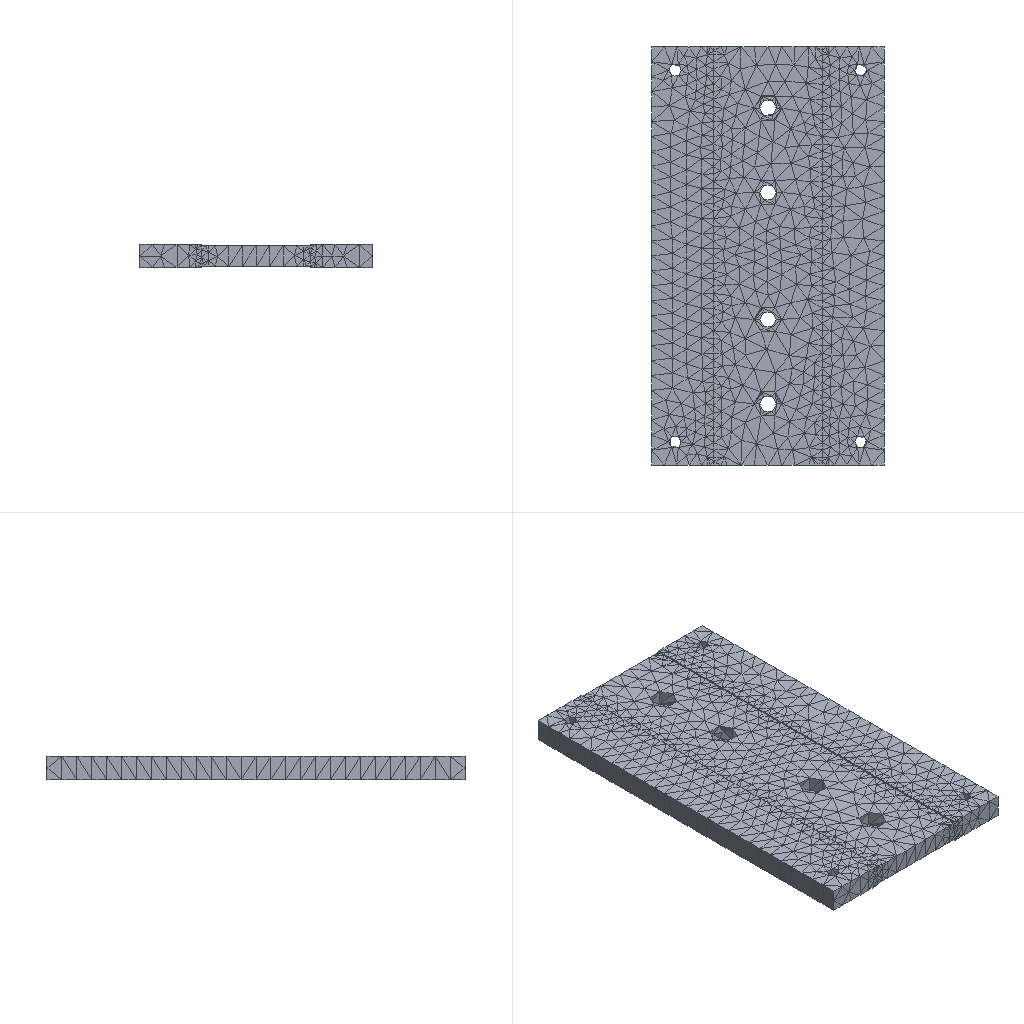Simulation study | ansys workbench
Set-up summary:
category,name,step,type,value,unit,region
solver,ansys_workbench
units,SI m-kg-s (Pa),,stated,"/units,MKS"
analysis,LS1,,static
load_step,LS1,LS1,static,nsubst=1; time=1
mesh,nodes,,,15924
mesh,elements,,,9787
element_type,SOLID187,,,9141
element_type,CONTA174,,,646
material,Structural Steel,,E,2e+11,Pa
material,Structural Steel,,nu,0.3
material,Structural Steel,,density,7850,kg m^-3
material,Structural Steel,,conductivity,60.5,W m^-1 C^-1
material,Structural Steel,,specific_heat,434,J kg^-1 C^-1
material,Structural Steel,,cte,1.2e-05,C^-1
material,Structural Steel,,permeability,10000
material,Structural Steel,,resistivity,1.7e-07,kg m^3 A^-2 s^-3
load,,LS1,moment,"1000 [dir=(0, 0, 1) n=3]",,all
bc,Fixed Supports,model,fixed,[dofs=ALL],,_FIXEDSU
contact,contact 1,,bonded (always),element=CONTA174
named_set,_FIXEDSU,,node,1510
Ansys APDL input file, long lists of numbers shortened:
/batch
/config,noeldb,1     ! force off writing results to database
*get,_wallstrt,active,,time,wall
! ANSYS input file written by Workbench version 2024 R1
! File used for geometry attach:
/title,wbnew--____ (A5)
! ****** Begin Custom Load Command Snippet ******
/COM, ACT Extensions:
/COM,     LSDYNA, 2024.1
/COM,/COM,     ANSYSMotion, 2024.1
/COM,
! ****** End   Custom Load Command Snippet ******
*DIM,_wb_ProjectScratch_dir,string,248
_wb_ProjectScratch_dir(1) = ''
*DIM,_wb_SolverFiles_dir,string,248
_wb_SolverFiles_dir(1) = ''
*DIM,_wb_userfiles_dir,string,248
_wb_userfiles_dir(1) = ''
/com,--- Data in consistent MKS units. See Solving Units in the help system for more information.
/units,MKS
/nopr
/wb,file,start              !  signify a WB generated input file
/prep7
! Turn off shape checking because checks already performed inside WB mesher.
! See help system for more information.
SHPP,OFF,,NOWARN
/nolist
etcon,set             ! allow ANSYS to choose best KEYOP's for 180x elements, resets any applicable keyopt to MAPDL defaults
/com,*********** Nodes for the whole assembly ***********
nblock,3,,17515
(1i9,3e20.9e3)
        1     4.000000000E-02    -2.700000000E-01    -1.400000000E-02
! (15922 more lines like these left out)
-1
/com,*********** Nodes for all Remote Points ***********
nblock,3
(1i9,3e20.9e3)
    15924     7.500000642E-02    -1.350000054E-01    -1.499999966E-02
-1
/wb,elem,start            !  set before creation of elements
/com,*********** Elements for Body 1 "SYS\GKZT-13-1.02.03.01.01_______" ***********
et,1,187
eblock,19,solid,,9141
(19i9)
        1        1        1        1        0        0        0        0       10        0        1     1619     2487     2246     2427    12549    15603    12547    12548
! (18281 more lines like these left out)
-1
/wb,elem,end               !  done creating elements
/com,*********** Send User Defined Coordinate System(s) ***********
csys,0
toffst,273.15,  ! Temperature offset from absolute zero
/com,*********** Set Reference Temperature ***********
tref,22.
/wb,mat,start              !  starting to send materials
/com,*********** Send Materials ***********
Temperature = 'TEMP' ! Temperature
MP,DENS,1,7850,	! kg m^-3
MP,ALPX,1,1.2e-05,	! C^-1
MP,C,1,434,	! J kg^-1 C^-1
MP,KXX,1,60.5,	! W m^-1 C^-1
MP,RSVX,1,1.7e-07,	! kg m^3 A^-2 s^-3
MP,EX,1,200000000000,	! Pa
MP,NUXY,1,0.3,
MP,MURX,1,10000,
/wb,mat,end                !  done sending materials
!************************* Model Summary ********************
!SYS\GKZT-13-1.02.03.01.01éæ¯å¨è¿æ¸¡é¡¶æ¿,	ç»æé¢,	matid,	1
!************************* End Model Summary ********************
! get the diagonal of the bounding box. Needed later for other things
*get,_xmin,node,,mnloc,x
*get,_ymin,node,,mnloc,y
*get,_zmin,node,,mnloc,z
*get,_xmax,node,,mxloc,x
*get,_ymax,node,,mxloc,y
*get,_zmax,node,,mxloc,z
_ASMDIAG=(_xmax-_xmin)*(_xmax-_xmin)+(_ymax-_ymin)*(_ymax-_ymin)+(_zmax-_zmin)*(_zmax-_zmin)
_ASMDIAG=SQRT(_ASMDIAG)
/wb,contact,start          !  starting to send contact
/wb,contact,end            !  done creating contacts
/golist
/wb,load,start             !  starting to send loads
/com,*********** Fixed Supports ***********
CMBLOCK,_FIXEDSU,NODE,     1510
(8i10)
        17        19        20        21        22        23        33        34
! (188 more lines like these left out)
cmsel,s,_FIXEDSU
d,all,all
nsel,all
/com,*********** Create Remote Point "ÄÚ²¿Ô¶³Ìµã" ***********
! -------- Remote Point Used by "Á¦¾Ø" --------
*set,tid,3
*set,cid,2
et,cid,174
et,tid,170
keyo,tid,2,1               ! Don't fix the pilot node
keyo,tid,4,111111
keyo,cid,12,5              ! Bonded Contact
keyo,cid,4,1               ! Deformable RBE3 style load
keyo,cid,2,2               ! MPC style contact
eblock,10,,,646
(15i9)
    12717        2        2        2        0     1470     1528     1510     1510    11580    11867     1510    11578
! (645 more lines like these left out)
-1
*set,_npilot,15924
_npilot43=_npilot
type,tid
mat ,cid
real,cid
tshape,pilo
en,13363,_npilot
tshape
/com,*********** Construct Moment Using Remote Attachment ***********
/gst,on,on
fini
*get,_numnode,node,0,count
*get,_numelem,elem,0,count
*get, _MAXELEMNUM, elem, 0, NUM, MAX
*get, _MAXNODENUM, node, 0, NUM, MAX
*get, _MAXELEMTYPE, etyp, 0, NUM, MAX
*get, _MAXREALCONST, rcon, 0, NUM, MAX
/go
/wb,load,end               !  done creating loads
/com,--- Number of total nodes = %_numnode%
/com,--- Number of contact elements = 646
/com,--- Number of spring elements = 0
/com,--- Number of bearing elements = 0
/com,--- Number of solid elements = 9141
/com,--- Number of condensed parts = 0
/com,--- Number of total elements = %_numelem%
*get,_wallbsol,active,,time,wall
/com,****************************************************************************
/com,*************************    SOLUTION       ********************************
/com,****************************************************************************
/solu
antype,0                   ! static analysis
_thickRatio=  1     ! Ratio of thick parts in the model
eqsl,pcg,1e-8,,,,,,1
cntr,print,1               ! print out contact info and also make no initial contact an error
cncheck,dmp		!	Enable program controlled contact splitting for distributed memory parallel run
dmpoption,emat,no             ! Don't combine emat file for DANSYS
dmpoption,esav,no             ! Don't combine esav file for DANSYS
nldiag,cont,iter           ! print out contact info each equilibrium iteration
rescontrol,,none                 ! Do not keep any restart files
/com,****************************************************
/com,******************* SOLVE FOR LS 1 OF 1 ****************
nsel,s,node,,15924
f,all,mx,0.
f,all,my,0.
f,all,mz,1000.
nsel,all
/nopr
/gopr
nsub,1,1,1
time,1.
outres,erase
outres,all,none
outres,nsol,all,
outres,rsol,all
outres,eangl,all
outres,etmp,all
outres,veng,all
outres,strs,all,
outres,epel,all,
outres,eppl,all,
outres,cont,all,
! *********** WB SOLVE COMMAND ***********
! check interactive state
*get,ANSINTER_,active,,int
*if,ANSINTER_,ne,0,then
/eof
*endif
solve
/com *************** Write FE CONNECTORS *********
CEWRITE,file,ce,,INTE
/com,****************************************************
/com,*************** FINISHED SOLVE FOR LS 1 *************
*get,_wallasol,active,,time,wall
/nopr
*get,_numnode,node,0,count
*get,_numelem,elem,0,count
*get, _MAXELEMNUM, elem, 0, NUM, MAX
*get, _MAXNODENUM, node, 0, NUM, MAX,,,INTERNAL
*get, _MAXELEMTYPE, etyp, 0, NUM, MAX
*get, _MAXREALCONST, rcon, 0, NUM, MAX
*get,_NSOLTHREADS,active,0,ntfs
*get,_NSOLPROCESSES,active,0,npfs
/gopr
*get,_PCGITER,active,,solu,cgiter
/post1
xmlo,ENCODING,ISO-8859-1
xmlo,parm
/xml,parm,xml
fini
/gopr
*get,_walldone,active,,time,wall
_preptime=(_wallbsol-_wallstrt)*3600
_solvtime=(_wallasol-_wallbsol)*3600
_posttime=(_walldone-_wallasol)*3600
_totaltim=(_walldone-_wallstrt)*3600
*get,_dlbratio,active,0,solu,dlbr
*get,_combtime,active,0,solu,comb
*get,_ssmode,active,0,solu,ssmm
*get,_ndofs,active,0,solu,ndof
*get,_sol_end_time,active,0,set,time
*if,_sol_end_time,eq,1.,then
/fclean				!clean distributed files
*endif
/com,--- Total number of nodes = %_numnode%
/com,--- Total number of elements = %_numelem%
/com,--- Element load balance ratio = %_dlbratio%
/com,--- Time to combine distributed files = %_combtime%
/com,--- Sparse memory mode = %_ssmode%
/com,--- Number of DOF = %_ndofs%
/wb,file,end               ! done with WB generated input
Results summary:
result,analyses[0].index,,,1
result,analyses[0].system,,,SYS
result,analyses[0].deck,,,deck.dat
result,analyses[0].solve_status,,,completed
result,analyses[0].analysis_type,,,static
result,analyses[0].physics,,,mechanical
result,analyses[0].unit_system,,,"MKS: m, kg, N, s, V, A, degC"
result,analyses[0].n_sets,,,1
result,analyses[0].load_steps[0].set,set=1,,1
result,analyses[0].load_steps[0].time_or_freq,set=1,,1
result,analyses[0].load_steps[0].max_displacement_magnitude,set=1,,2.39164e-07
result,analyses[0].load_steps[0].max_von_mises_nodal,set=1,,6.32605e+06
result,analyses[0].load_steps[0].reaction_force_sum_xyz[1],set=1,,4.52484e-07
result,analyses[0].load_steps[0].reaction_force_sum_xyz[2],set=1,,5.77748e-07
result,analyses[0].load_steps[0].reaction_force_sum_xyz[3],set=1,,1.49301e-06
result,geometry_export[0][0],,,.step
result,geometry_export[0][1],,,ok
result,geometry_export[0][2],,,1